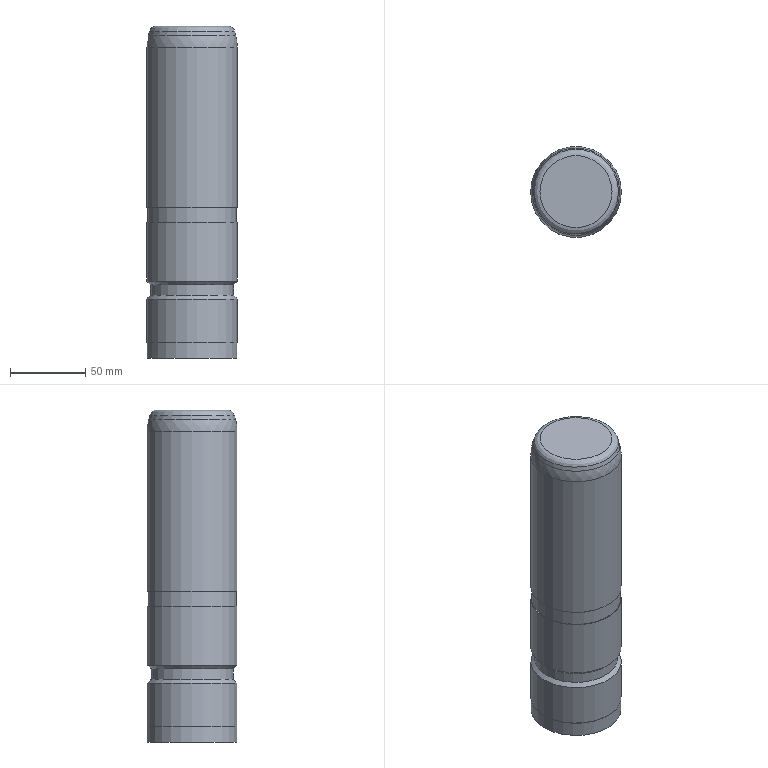Part | NX | features solid 2 | 1 solid | 16 faces | box 60 x 60 x 220 mm | volume 613364 mm3 | cylinder 6 | plane 5 | cone 3 | torus 1 | sphere 1 | commonest cylinder face diameters 60 x3 55 x1 59 x1 59.5 x1
STEP:
#1=CARTESIAN_POINT('',(-1234.5,125.,-150.));
#2=VERTEX_POINT('',#1);
#3=CARTESIAN_POINT('',(-1205.,125.,-150.));
#4=DIRECTION('',(0.,0.,-1.));
#5=DIRECTION('',(-1.,0.,0.));
#6=AXIS2_PLACEMENT_3D('',#3,#4,#5);
#7=CIRCLE('',#6,29.5);
#8=EDGE_CURVE('',#2,#2,#7,.T.);
#9=ORIENTED_EDGE('',*,*,#8,.F.);
#10=EDGE_LOOP('',(#9));
#11=FACE_BOUND('',#10,.T.);
#12=CARTESIAN_POINT('',(-1235.,125.,-150.));
#13=VERTEX_POINT('',#12);
#14=CARTESIAN_POINT('',(-1205.,125.,-150.));
#15=DIRECTION('',(0.,0.,-1.));
#16=DIRECTION('',(-1.,0.,0.));
#17=AXIS2_PLACEMENT_3D('',#14,#15,#16);
#18=CIRCLE('',#17,30.);
#19=EDGE_CURVE('',#13,#13,#18,.F.);
#20=ORIENTED_EDGE('',*,*,#19,.F.);
#21=EDGE_LOOP('',(#20));
#22=FACE_BOUND('',#21,.T.);
#23=CARTESIAN_POINT('',(-1300.,255.,-150.));
#24=DIRECTION('',(0.,0.,-1.));
#25=DIRECTION('',(-1.,0.,0.));
#26=AXIS2_PLACEMENT_3D('',#23,#24,#25);
#27=PLANE('',#26);
#28=ADVANCED_FACE('',(#11,#22),#27,.T.);
#29=CARTESIAN_POINT('',(-1181.132,125.,-30.));
#30=VERTEX_POINT('',#29);
#31=CARTESIAN_POINT('',(-1205.,125.,-30.));
#32=DIRECTION('',(0.,0.,1.));
#33=DIRECTION('',(1.,0.,0.));
#34=AXIS2_PLACEMENT_3D('',#31,#32,#33);
#35=CIRCLE('',#34,23.868);
#36=EDGE_CURVE('',#30,#30,#35,.T.);
#37=ORIENTED_EDGE('',*,*,#36,.T.);
#38=EDGE_LOOP('',(#37));
#39=FACE_BOUND('',#38,.T.);
#40=CARTESIAN_POINT('',(-1205.,125.,-30.));
#41=DIRECTION('',(0.,0.,1.));
#42=DIRECTION('',(1.,0.,0.));
#43=AXIS2_PLACEMENT_3D('',#40,#41,#42);
#44=PLANE('',#43);
#45=ADVANCED_FACE('',(#39),#44,.T.);
#46=ORIENTED_EDGE('',*,*,#36,.F.);
#47=EDGE_LOOP('',(#46));
#48=FACE_BOUND('',#47,.T.);
#49=CARTESIAN_POINT('',(-1176.786,125.,-33.335));
#50=VERTEX_POINT('',#49);
#51=CARTESIAN_POINT('',(-1205.,125.,-33.335));
#52=DIRECTION('',(0.,0.,1.));
#53=DIRECTION('',(1.,0.,0.));
#54=AXIS2_PLACEMENT_3D('',#51,#52,#53);
#55=CIRCLE('',#54,28.214);
#56=EDGE_CURVE('',#50,#50,#55,.F.);
#57=ORIENTED_EDGE('',*,*,#56,.F.);
#58=EDGE_LOOP('',(#57));
#59=FACE_BOUND('',#58,.T.);
#60=CARTESIAN_POINT('',(-1205.,125.,-34.5));
#61=DIRECTION('',(0.,0.,1.));
#62=DIRECTION('',(1.,0.,0.));
#63=AXIS2_PLACEMENT_3D('',#60,#61,#62);
#64=TOROIDAL_SURFACE('',#63,23.868,4.5);
#65=ADVANCED_FACE('',(#48,#59),#64,.T.);
#66=ORIENTED_EDGE('',*,*,#56,.T.);
#67=EDGE_LOOP('',(#66));
#68=FACE_BOUND('',#67,.T.);
#69=CARTESIAN_POINT('',(-1233.978,125.,-36.185));
#70=VERTEX_POINT('',#69);
#71=CARTESIAN_POINT('',(-1205.,125.,-36.185));
#72=DIRECTION('',(0.,0.,-1.));
#73=DIRECTION('',(-1.,0.,0.));
#74=AXIS2_PLACEMENT_3D('',#71,#72,#73);
#75=CIRCLE('',#74,28.978);
#76=EDGE_CURVE('',#70,#70,#75,.F.);
#77=ORIENTED_EDGE('',*,*,#76,.T.);
#78=EDGE_LOOP('',(#77));
#79=FACE_BOUND('',#78,.T.);
#80=CARTESIAN_POINT('',(-1205.,125.,-30.));
#81=DIRECTION('',(0.,0.,-1.));
#82=DIRECTION('',(-1.,0.,0.));
#83=AXIS2_PLACEMENT_3D('',#80,#81,#82);
#84=CONICAL_SURFACE('',#83,27.32,0.2618);
#85=ADVANCED_FACE('',(#68,#79),#84,.T.);
#86=ORIENTED_EDGE('',*,*,#76,.F.);
#87=EDGE_LOOP('',(#86));
#88=FACE_BOUND('',#87,.T.);
#89=CARTESIAN_POINT('',(-1175.,125.,-43.95));
#90=VERTEX_POINT('',#89);
#91=CARTESIAN_POINT('',(-1205.,125.,-43.95));
#92=DIRECTION('',(0.,0.,1.));
#93=DIRECTION('',(1.,0.,0.));
#94=AXIS2_PLACEMENT_3D('',#91,#92,#93);
#95=CIRCLE('',#94,30.);
#96=EDGE_CURVE('',#90,#90,#95,.F.);
#97=ORIENTED_EDGE('',*,*,#96,.F.);
#98=EDGE_LOOP('',(#97));
#99=FACE_BOUND('',#98,.T.);
#100=CARTESIAN_POINT('',(-1205.,125.,-43.95));
#101=DIRECTION('',(0.,0.,1.));
#102=DIRECTION('',(1.,0.,0.));
#103=AXIS2_PLACEMENT_3D('',#100,#101,#102);
#104=SPHERICAL_SURFACE('',#103,30.);
#105=ADVANCED_FACE('',(#88,#99),#104,.T.);
#106=ORIENTED_EDGE('',*,*,#19,.T.);
#107=EDGE_LOOP('',(#106));
#108=FACE_BOUND('',#107,.T.);
#109=ORIENTED_EDGE('',*,*,#96,.T.);
#110=EDGE_LOOP('',(#109));
#111=FACE_BOUND('',#110,.T.);
#112=CARTESIAN_POINT('',(-1205.,125.,-180.));
#113=DIRECTION('',(0.,0.,1.));
#114=DIRECTION('',(1.,0.,0.));
#115=AXIS2_PLACEMENT_3D('',#112,#113,#114);
#116=CYLINDRICAL_SURFACE('',#115,30.);
#117=ADVANCED_FACE('',(#108,#111),#116,.T.);
#118=CARTESIAN_POINT('',(-1232.5,125.,-201.5));
#119=VERTEX_POINT('',#118);
#120=CARTESIAN_POINT('',(-1205.,125.,-201.5));
#121=DIRECTION('',(0.,0.,-1.));
#122=DIRECTION('',(-1.,0.,0.));
#123=AXIS2_PLACEMENT_3D('',#120,#121,#122);
#124=CIRCLE('',#123,27.5);
#125=EDGE_CURVE('',#119,#119,#124,.T.);
#126=ORIENTED_EDGE('',*,*,#125,.F.);
#127=EDGE_LOOP('',(#126));
#128=FACE_BOUND('',#127,.T.);
#129=CARTESIAN_POINT('',(-1175.,125.,-199.));
#130=VERTEX_POINT('',#129);
#131=CARTESIAN_POINT('',(-1205.,125.,-199.));
#132=DIRECTION('',(0.,0.,1.));
#133=DIRECTION('',(1.,0.,0.));
#134=AXIS2_PLACEMENT_3D('',#131,#132,#133);
#135=CIRCLE('',#134,30.);
#136=EDGE_CURVE('',#130,#130,#135,.T.);
#137=ORIENTED_EDGE('',*,*,#136,.F.);
#138=EDGE_LOOP('',(#137));
#139=FACE_BOUND('',#138,.T.);
#140=CARTESIAN_POINT('',(-1205.,125.,-201.5));
#141=DIRECTION('',(0.,0.,1.));
#142=DIRECTION('',(1.,0.,0.));
#143=AXIS2_PLACEMENT_3D('',#140,#141,#142);
#144=CONICAL_SURFACE('',#143,27.5,0.7854);
#145=ADVANCED_FACE('',(#128,#139),#144,.T.);
#146=ORIENTED_EDGE('',*,*,#125,.T.);
#147=EDGE_LOOP('',(#146));
#148=FACE_BOUND('',#147,.T.);
#149=CARTESIAN_POINT('',(-1232.5,125.,-208.5));
#150=VERTEX_POINT('',#149);
#151=CARTESIAN_POINT('',(-1205.,125.,-208.5));
#152=DIRECTION('',(0.,0.,-1.));
#153=DIRECTION('',(-1.,0.,0.));
#154=AXIS2_PLACEMENT_3D('',#151,#152,#153);
#155=CIRCLE('',#154,27.5);
#156=EDGE_CURVE('',#150,#150,#155,.T.);
#157=ORIENTED_EDGE('',*,*,#156,.F.);
#158=EDGE_LOOP('',(#157));
#159=FACE_BOUND('',#158,.T.);
#160=CARTESIAN_POINT('',(-1205.,125.,-208.5));
#161=DIRECTION('',(0.,0.,1.));
#162=DIRECTION('',(1.,0.,0.));
#163=AXIS2_PLACEMENT_3D('',#160,#161,#162);
#164=CYLINDRICAL_SURFACE('',#163,27.5);
#165=ADVANCED_FACE('',(#148,#159),#164,.T.);
#166=CARTESIAN_POINT('',(-1175.5,125.,-160.));
#167=VERTEX_POINT('',#166);
#168=CARTESIAN_POINT('',(-1205.,125.,-160.));
#169=DIRECTION('',(0.,0.,1.));
#170=DIRECTION('',(1.,0.,0.));
#171=AXIS2_PLACEMENT_3D('',#168,#169,#170);
#172=CIRCLE('',#171,29.5);
#173=EDGE_CURVE('',#167,#167,#172,.T.);
#174=ORIENTED_EDGE('',*,*,#173,.F.);
#175=EDGE_LOOP('',(#174));
#176=FACE_BOUND('',#175,.T.);
#177=CARTESIAN_POINT('',(-1235.,125.,-160.));
#178=VERTEX_POINT('',#177);
#179=CARTESIAN_POINT('',(-1205.,125.,-160.));
#180=DIRECTION('',(0.,0.,-1.));
#181=DIRECTION('',(-1.,0.,0.));
#182=AXIS2_PLACEMENT_3D('',#179,#180,#181);
#183=CIRCLE('',#182,30.);
#184=EDGE_CURVE('',#178,#178,#183,.T.);
#185=ORIENTED_EDGE('',*,*,#184,.F.);
#186=EDGE_LOOP('',(#185));
#187=FACE_BOUND('',#186,.T.);
#188=CARTESIAN_POINT('',(-1205.,125.,-160.));
#189=DIRECTION('',(0.,0.,1.));
#190=DIRECTION('',(1.,0.,0.));
#191=AXIS2_PLACEMENT_3D('',#188,#189,#190);
#192=PLANE('',#191);
#193=ADVANCED_FACE('',(#176,#187),#192,.T.);
#194=ORIENTED_EDGE('',*,*,#184,.T.);
#195=EDGE_LOOP('',(#194));
#196=FACE_BOUND('',#195,.T.);
#197=ORIENTED_EDGE('',*,*,#136,.T.);
#198=EDGE_LOOP('',(#197));
#199=FACE_BOUND('',#198,.T.);
#200=CARTESIAN_POINT('',(-1205.,125.,-199.));
#201=DIRECTION('',(0.,0.,1.));
#202=DIRECTION('',(1.,0.,0.));
#203=AXIS2_PLACEMENT_3D('',#200,#201,#202);
#204=CYLINDRICAL_SURFACE('',#203,30.);
#205=ADVANCED_FACE('',(#196,#199),#204,.T.);
#206=ORIENTED_EDGE('',*,*,#8,.T.);
#207=EDGE_LOOP('',(#206));
#208=FACE_BOUND('',#207,.T.);
#209=ORIENTED_EDGE('',*,*,#173,.T.);
#210=EDGE_LOOP('',(#209));
#211=FACE_BOUND('',#210,.T.);
#212=CARTESIAN_POINT('',(-1205.,125.,-160.));
#213=DIRECTION('',(0.,0.,1.));
#214=DIRECTION('',(1.,0.,0.));
#215=AXIS2_PLACEMENT_3D('',#212,#213,#214);
#216=CYLINDRICAL_SURFACE('',#215,29.5);
#217=ADVANCED_FACE('',(#208,#211),#216,.T.);
#218=CARTESIAN_POINT('',(-1234.75,125.,-240.));
#219=VERTEX_POINT('',#218);
#220=CARTESIAN_POINT('',(-1205.,125.,-240.));
#221=DIRECTION('',(0.,0.,-1.));
#222=DIRECTION('',(-1.,0.,0.));
#223=AXIS2_PLACEMENT_3D('',#220,#221,#222);
#224=CIRCLE('',#223,29.75);
#225=EDGE_CURVE('',#219,#219,#224,.T.);
#226=ORIENTED_EDGE('',*,*,#225,.F.);
#227=EDGE_LOOP('',(#226));
#228=FACE_BOUND('',#227,.T.);
#229=CARTESIAN_POINT('',(-1175.,125.,-240.));
#230=VERTEX_POINT('',#229);
#231=CARTESIAN_POINT('',(-1205.,125.,-240.));
#232=DIRECTION('',(0.,0.,1.));
#233=DIRECTION('',(1.,0.,0.));
#234=AXIS2_PLACEMENT_3D('',#231,#232,#233);
#235=CIRCLE('',#234,30.);
#236=EDGE_CURVE('',#230,#230,#235,.T.);
#237=ORIENTED_EDGE('',*,*,#236,.F.);
#238=EDGE_LOOP('',(#237));
#239=FACE_BOUND('',#238,.T.);
#240=CARTESIAN_POINT('',(-1205.,125.,-240.));
#241=DIRECTION('',(0.,0.,-1.));
#242=DIRECTION('',(-1.,0.,0.));
#243=AXIS2_PLACEMENT_3D('',#240,#241,#242);
#244=PLANE('',#243);
#245=ADVANCED_FACE('',(#228,#239),#244,.T.);
#246=CARTESIAN_POINT('',(-1175.,125.,-211.));
#247=VERTEX_POINT('',#246);
#248=CARTESIAN_POINT('',(-1205.,125.,-211.));
#249=DIRECTION('',(0.,0.,1.));
#250=DIRECTION('',(1.,0.,0.));
#251=AXIS2_PLACEMENT_3D('',#248,#249,#250);
#252=CIRCLE('',#251,30.);
#253=EDGE_CURVE('',#247,#247,#252,.T.);
#254=ORIENTED_EDGE('',*,*,#253,.F.);
#255=EDGE_LOOP('',(#254));
#256=FACE_BOUND('',#255,.T.);
#257=ORIENTED_EDGE('',*,*,#236,.T.);
#258=EDGE_LOOP('',(#257));
#259=FACE_BOUND('',#258,.T.);
#260=CARTESIAN_POINT('',(-1205.,125.,-240.));
#261=DIRECTION('',(0.,0.,1.));
#262=DIRECTION('',(1.,0.,0.));
#263=AXIS2_PLACEMENT_3D('',#260,#261,#262);
#264=CYLINDRICAL_SURFACE('',#263,30.);
#265=ADVANCED_FACE('',(#256,#259),#264,.T.);
#266=CARTESIAN_POINT('',(-1175.25,125.,-250.));
#267=VERTEX_POINT('',#266);
#268=CARTESIAN_POINT('',(-1205.,125.,-250.));
#269=DIRECTION('',(0.,0.,1.));
#270=DIRECTION('',(1.,0.,0.));
#271=AXIS2_PLACEMENT_3D('',#268,#269,#270);
#272=CIRCLE('',#271,29.75);
#273=EDGE_CURVE('',#267,#267,#272,.T.);
#274=ORIENTED_EDGE('',*,*,#273,.F.);
#275=EDGE_LOOP('',(#274));
#276=FACE_BOUND('',#275,.T.);
#277=CARTESIAN_POINT('',(-1205.,125.,-250.));
#278=DIRECTION('',(0.,0.,-1.));
#279=DIRECTION('',(-1.,0.,0.));
#280=AXIS2_PLACEMENT_3D('',#277,#278,#279);
#281=PLANE('',#280);
#282=ADVANCED_FACE('',(#276),#281,.T.);
#283=ORIENTED_EDGE('',*,*,#225,.T.);
#284=EDGE_LOOP('',(#283));
#285=FACE_BOUND('',#284,.T.);
#286=ORIENTED_EDGE('',*,*,#273,.T.);
#287=EDGE_LOOP('',(#286));
#288=FACE_BOUND('',#287,.T.);
#289=CARTESIAN_POINT('',(-1205.,125.,-250.));
#290=DIRECTION('',(0.,0.,1.));
#291=DIRECTION('',(1.,0.,0.));
#292=AXIS2_PLACEMENT_3D('',#289,#290,#291);
#293=CYLINDRICAL_SURFACE('',#292,29.75);
#294=ADVANCED_FACE('',(#285,#288),#293,.T.);
#295=ORIENTED_EDGE('',*,*,#253,.T.);
#296=EDGE_LOOP('',(#295));
#297=FACE_BOUND('',#296,.T.);
#298=ORIENTED_EDGE('',*,*,#156,.T.);
#299=EDGE_LOOP('',(#298));
#300=FACE_BOUND('',#299,.T.);
#301=CARTESIAN_POINT('',(-1205.,125.,-208.5));
#302=DIRECTION('',(0.,0.,-1.));
#303=DIRECTION('',(-1.,0.,0.));
#304=AXIS2_PLACEMENT_3D('',#301,#302,#303);
#305=CONICAL_SURFACE('',#304,27.5,0.7854);
#306=ADVANCED_FACE('',(#297,#300),#305,.T.);
#307=CLOSED_SHELL('',(#28,#45,#65,#85,#105,#117,#145,#165,#193,#205,#217,#245,#265,#282,#294,#306));
#308=MANIFOLD_SOLID_BREP('',#307);
#309=(LENGTH_UNIT()NAMED_UNIT(*)SI_UNIT(.MILLI.,.METRE.));
#310=UNCERTAINTY_MEASURE_WITH_UNIT(LENGTH_MEASURE(0.00001),#309,'','');
#311=(NAMED_UNIT(*)PLANE_ANGLE_UNIT()SI_UNIT($,.RADIAN.));
#312=(NAMED_UNIT(*)SI_UNIT($,.STERADIAN.)SOLID_ANGLE_UNIT());
#313=(GEOMETRIC_REPRESENTATION_CONTEXT(3)GLOBAL_UNCERTAINTY_ASSIGNED_CONTEXT((#310))GLOBAL_UNIT_ASSIGNED_CONTEXT((#309,#311,#312))REPRESENTATION_CONTEXT('',''));
#314=ADVANCED_BREP_SHAPE_REPRESENTATION('',(#308),#313);